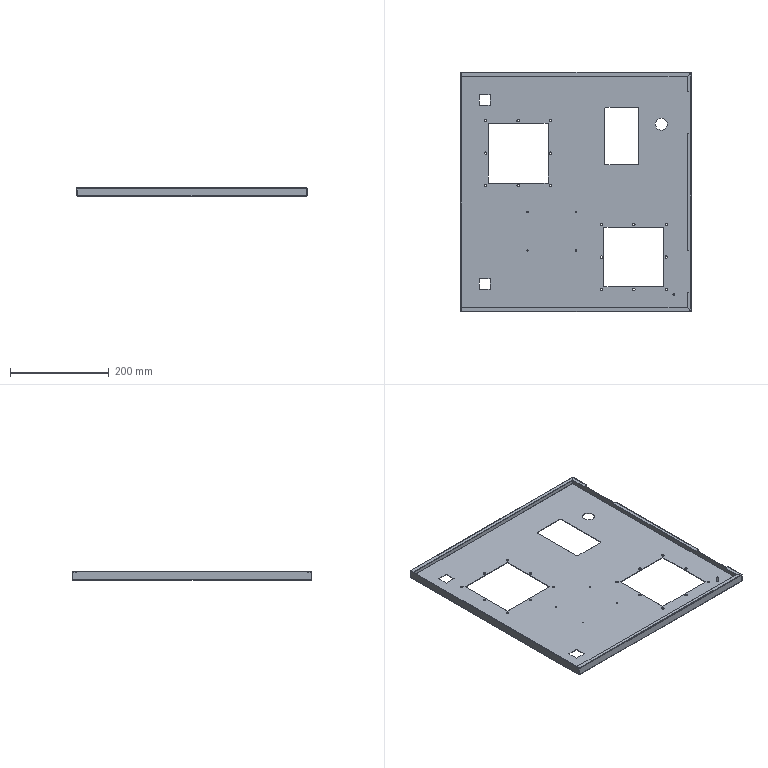Part | STEP file | 1 solid | 169 faces | box 465 x 484 x 17 mm | volume 267277 mm3 | plane 91 | cylinder 70 | spline 8 | commonest cylinder face diameters 5 x32 0.02 x9 2.42 x9 2.5 x8 2 x4 4 x4